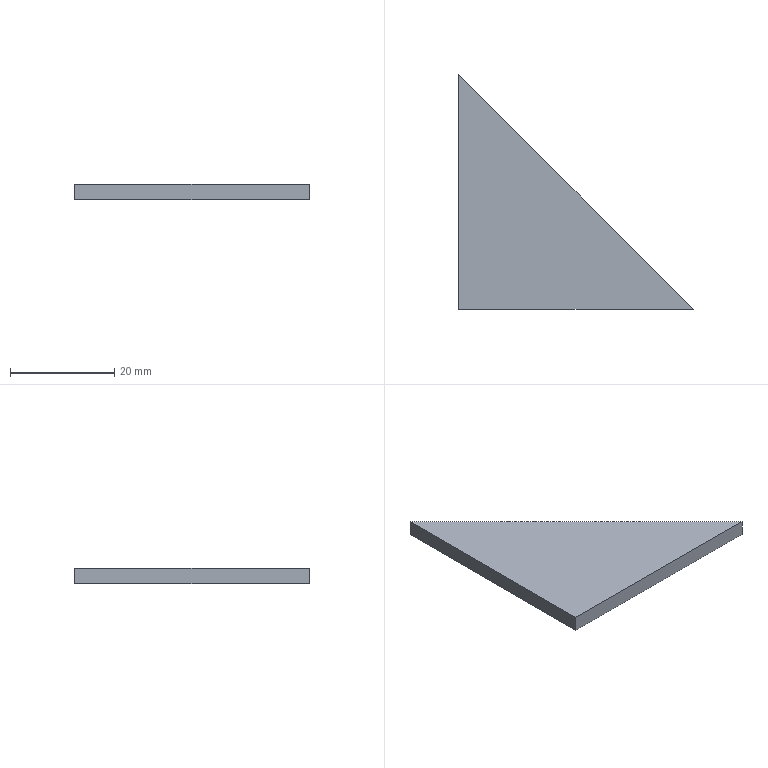Part | STEP file | 5090108 | 1 solid | 5 faces | box 45 x 45 x 3 mm | volume 3037 mm3 | plane 5
STEP:
#1=CARTESIAN_POINT('',(0.,0.,0.));
#2=DIRECTION('',(0.,0.,1.));
#3=DIRECTION('',(1.,0.,0.));
#4=AXIS2_PLACEMENT_3D('',#1,#2,#3);
#5=CARTESIAN_POINT('',(-8.721,-36.279,0.));
#6=VERTEX_POINT('',#5);
#7=CARTESIAN_POINT('',(36.279,-36.279,0.));
#8=VERTEX_POINT('',#7);
#9=CARTESIAN_POINT('',(-8.721,-36.279,0.));
#10=DIRECTION('',(1.,0.,0.));
#11=VECTOR('',#10,1.);
#12=LINE('',#9,#11);
#13=CARTESIAN_POINT('',(-8.721,-36.279,3.));
#14=DIRECTION('',(0.,1.,0.));
#15=DIRECTION('',(0.,0.,1.));
#16=AXIS2_PLACEMENT_3D('',#13,#14,#15);
#17=PLANE('',#16);
#18=CARTESIAN_POINT('',(-3.,0.));
#19=DIRECTION('',(0.,1.));
#20=VECTOR('',#19,1.);
#21=LINE('',#18,#20);
#22=(GEOMETRIC_REPRESENTATION_CONTEXT(2)PARAMETRIC_REPRESENTATION_CONTEXT()REPRESENTATION_CONTEXT('',''));
#23=DEFINITIONAL_REPRESENTATION('',(#21),#22);
#24=PCURVE('',#17,#23);
#25=CARTESIAN_POINT('',(0.,0.,0.));
#26=DIRECTION('',(0.,0.,-1.));
#27=DIRECTION('',(-1.,0.,0.));
#28=AXIS2_PLACEMENT_3D('',#25,#26,#27);
#29=PLANE('',#28);
#30=CARTESIAN_POINT('',(8.721,-36.279));
#31=DIRECTION('',(-1.,0.));
#32=VECTOR('',#31,1.);
#33=LINE('',#30,#32);
#34=(GEOMETRIC_REPRESENTATION_CONTEXT(2)PARAMETRIC_REPRESENTATION_CONTEXT()REPRESENTATION_CONTEXT('',''));
#35=DEFINITIONAL_REPRESENTATION('',(#33),#34);
#36=PCURVE('',#29,#35);
#37=SURFACE_CURVE('',#12,(#24,#36),.PCURVE_S1.);
#38=EDGE_CURVE('',#6,#8,#37,.T.);
#39=ORIENTED_EDGE('',*,*,#38,.T.);
#40=CARTESIAN_POINT('',(36.279,-36.279,3.));
#41=VERTEX_POINT('',#40);
#42=CARTESIAN_POINT('',(36.279,-36.279,3.));
#43=DIRECTION('',(0.,0.,-1.));
#44=VECTOR('',#43,1.);
#45=LINE('',#42,#44);
#46=CARTESIAN_POINT('',(0.,45.));
#47=DIRECTION('',(-1.,0.));
#48=VECTOR('',#47,1.);
#49=LINE('',#46,#48);
#50=(GEOMETRIC_REPRESENTATION_CONTEXT(2)PARAMETRIC_REPRESENTATION_CONTEXT()REPRESENTATION_CONTEXT('',''));
#51=DEFINITIONAL_REPRESENTATION('',(#49),#50);
#52=PCURVE('',#17,#51);
#53=CARTESIAN_POINT('',(-8.721,8.721,3.));
#54=DIRECTION('',(-0.7071,-0.7071,0.));
#55=DIRECTION('',(0.7071,-0.7071,0.));
#56=AXIS2_PLACEMENT_3D('',#53,#54,#55);
#57=PLANE('',#56);
#58=CARTESIAN_POINT('',(63.64,0.));
#59=DIRECTION('',(0.,-1.));
#60=VECTOR('',#59,1.);
#61=LINE('',#58,#60);
#62=(GEOMETRIC_REPRESENTATION_CONTEXT(2)PARAMETRIC_REPRESENTATION_CONTEXT()REPRESENTATION_CONTEXT('',''));
#63=DEFINITIONAL_REPRESENTATION('',(#61),#62);
#64=PCURVE('',#57,#63);
#65=SURFACE_CURVE('',#45,(#52,#64),.PCURVE_S1.);
#66=EDGE_CURVE('',#41,#8,#65,.T.);
#67=ORIENTED_EDGE('',*,*,#66,.F.);
#68=CARTESIAN_POINT('',(-8.721,-36.279,3.));
#69=VERTEX_POINT('',#68);
#70=CARTESIAN_POINT('',(-8.721,-36.279,3.));
#71=DIRECTION('',(1.,0.,0.));
#72=VECTOR('',#71,1.);
#73=LINE('',#70,#72);
#74=CARTESIAN_POINT('',(0.,0.));
#75=DIRECTION('',(0.,1.));
#76=VECTOR('',#75,1.);
#77=LINE('',#74,#76);
#78=(GEOMETRIC_REPRESENTATION_CONTEXT(2)PARAMETRIC_REPRESENTATION_CONTEXT()REPRESENTATION_CONTEXT('',''));
#79=DEFINITIONAL_REPRESENTATION('',(#77),#78);
#80=PCURVE('',#17,#79);
#81=CARTESIAN_POINT('',(0.,0.,3.));
#82=DIRECTION('',(0.,0.,-1.));
#83=DIRECTION('',(-1.,0.,0.));
#84=AXIS2_PLACEMENT_3D('',#81,#82,#83);
#85=PLANE('',#84);
#86=CARTESIAN_POINT('',(8.721,-36.279));
#87=DIRECTION('',(-1.,0.));
#88=VECTOR('',#87,1.);
#89=LINE('',#86,#88);
#90=(GEOMETRIC_REPRESENTATION_CONTEXT(2)PARAMETRIC_REPRESENTATION_CONTEXT()REPRESENTATION_CONTEXT('',''));
#91=DEFINITIONAL_REPRESENTATION('',(#89),#90);
#92=PCURVE('',#85,#91);
#93=SURFACE_CURVE('',#73,(#80,#92),.PCURVE_S1.);
#94=EDGE_CURVE('',#69,#41,#93,.T.);
#95=ORIENTED_EDGE('',*,*,#94,.F.);
#96=CARTESIAN_POINT('',(-8.721,-36.279,3.));
#97=DIRECTION('',(0.,0.,-1.));
#98=VECTOR('',#97,1.);
#99=LINE('',#96,#98);
#100=CARTESIAN_POINT('',(0.,0.));
#101=DIRECTION('',(-1.,0.));
#102=VECTOR('',#101,1.);
#103=LINE('',#100,#102);
#104=(GEOMETRIC_REPRESENTATION_CONTEXT(2)PARAMETRIC_REPRESENTATION_CONTEXT()REPRESENTATION_CONTEXT('',''));
#105=DEFINITIONAL_REPRESENTATION('',(#103),#104);
#106=PCURVE('',#17,#105);
#107=CARTESIAN_POINT('',(-8.721,8.721,3.));
#108=DIRECTION('',(1.,0.,0.));
#109=DIRECTION('',(0.,1.,0.));
#110=AXIS2_PLACEMENT_3D('',#107,#108,#109);
#111=PLANE('',#110);
#112=CARTESIAN_POINT('',(-45.,0.));
#113=DIRECTION('',(0.,-1.));
#114=VECTOR('',#113,1.);
#115=LINE('',#112,#114);
#116=(GEOMETRIC_REPRESENTATION_CONTEXT(2)PARAMETRIC_REPRESENTATION_CONTEXT()REPRESENTATION_CONTEXT('',''));
#117=DEFINITIONAL_REPRESENTATION('',(#115),#116);
#118=PCURVE('',#111,#117);
#119=SURFACE_CURVE('',#99,(#106,#118),.PCURVE_S1.);
#120=EDGE_CURVE('',#69,#6,#119,.T.);
#121=ORIENTED_EDGE('',*,*,#120,.T.);
#122=EDGE_LOOP('',(#39,#67,#95,#121));
#123=FACE_BOUND('',#122,.T.);
#124=ADVANCED_FACE('',(#123),#17,.F.);
#125=CARTESIAN_POINT('',(-8.721,8.721,0.));
#126=VERTEX_POINT('',#125);
#127=CARTESIAN_POINT('',(-8.721,8.721,0.));
#128=DIRECTION('',(-0.7071,0.7071,0.));
#129=VECTOR('',#128,1.);
#130=LINE('',#127,#129);
#131=CARTESIAN_POINT('',(0.,-3.));
#132=DIRECTION('',(-1.,0.));
#133=VECTOR('',#132,1.);
#134=LINE('',#131,#133);
#135=(GEOMETRIC_REPRESENTATION_CONTEXT(2)PARAMETRIC_REPRESENTATION_CONTEXT()REPRESENTATION_CONTEXT('',''));
#136=DEFINITIONAL_REPRESENTATION('',(#134),#135);
#137=PCURVE('',#57,#136);
#138=CARTESIAN_POINT('',(8.721,8.721));
#139=DIRECTION('',(0.7071,0.7071));
#140=VECTOR('',#139,1.);
#141=LINE('',#138,#140);
#142=(GEOMETRIC_REPRESENTATION_CONTEXT(2)PARAMETRIC_REPRESENTATION_CONTEXT()REPRESENTATION_CONTEXT('',''));
#143=DEFINITIONAL_REPRESENTATION('',(#141),#142);
#144=PCURVE('',#29,#143);
#145=SURFACE_CURVE('',#130,(#137,#144),.PCURVE_S1.);
#146=EDGE_CURVE('',#8,#126,#145,.T.);
#147=ORIENTED_EDGE('',*,*,#146,.T.);
#148=CARTESIAN_POINT('',(-8.721,8.721,3.));
#149=VERTEX_POINT('',#148);
#150=CARTESIAN_POINT('',(-8.721,8.721,3.));
#151=DIRECTION('',(0.,0.,-1.));
#152=VECTOR('',#151,1.);
#153=LINE('',#150,#152);
#154=CARTESIAN_POINT('',(0.,0.));
#155=DIRECTION('',(0.,-1.));
#156=VECTOR('',#155,1.);
#157=LINE('',#154,#156);
#158=(GEOMETRIC_REPRESENTATION_CONTEXT(2)PARAMETRIC_REPRESENTATION_CONTEXT()REPRESENTATION_CONTEXT('',''));
#159=DEFINITIONAL_REPRESENTATION('',(#157),#158);
#160=PCURVE('',#57,#159);
#161=CARTESIAN_POINT('',(0.,0.));
#162=DIRECTION('',(0.,-1.));
#163=VECTOR('',#162,1.);
#164=LINE('',#161,#163);
#165=(GEOMETRIC_REPRESENTATION_CONTEXT(2)PARAMETRIC_REPRESENTATION_CONTEXT()REPRESENTATION_CONTEXT('',''));
#166=DEFINITIONAL_REPRESENTATION('',(#164),#165);
#167=PCURVE('',#111,#166);
#168=SURFACE_CURVE('',#153,(#160,#167),.PCURVE_S1.);
#169=EDGE_CURVE('',#149,#126,#168,.T.);
#170=ORIENTED_EDGE('',*,*,#169,.F.);
#171=CARTESIAN_POINT('',(-8.721,8.721,3.));
#172=DIRECTION('',(-0.7071,0.7071,0.));
#173=VECTOR('',#172,1.);
#174=LINE('',#171,#173);
#175=CARTESIAN_POINT('',(0.,0.));
#176=DIRECTION('',(-1.,0.));
#177=VECTOR('',#176,1.);
#178=LINE('',#175,#177);
#179=(GEOMETRIC_REPRESENTATION_CONTEXT(2)PARAMETRIC_REPRESENTATION_CONTEXT()REPRESENTATION_CONTEXT('',''));
#180=DEFINITIONAL_REPRESENTATION('',(#178),#179);
#181=PCURVE('',#57,#180);
#182=CARTESIAN_POINT('',(8.721,8.721));
#183=DIRECTION('',(0.7071,0.7071));
#184=VECTOR('',#183,1.);
#185=LINE('',#182,#184);
#186=(GEOMETRIC_REPRESENTATION_CONTEXT(2)PARAMETRIC_REPRESENTATION_CONTEXT()REPRESENTATION_CONTEXT('',''));
#187=DEFINITIONAL_REPRESENTATION('',(#185),#186);
#188=PCURVE('',#85,#187);
#189=SURFACE_CURVE('',#174,(#181,#188),.PCURVE_S1.);
#190=EDGE_CURVE('',#41,#149,#189,.T.);
#191=ORIENTED_EDGE('',*,*,#190,.F.);
#192=ORIENTED_EDGE('',*,*,#66,.T.);
#193=EDGE_LOOP('',(#147,#170,#191,#192));
#194=FACE_BOUND('',#193,.T.);
#195=ADVANCED_FACE('',(#194),#57,.F.);
#196=CARTESIAN_POINT('',(-8.721,8.721,0.));
#197=DIRECTION('',(0.,-1.,0.));
#198=VECTOR('',#197,1.);
#199=LINE('',#196,#198);
#200=CARTESIAN_POINT('',(0.,-3.));
#201=DIRECTION('',(-1.,0.));
#202=VECTOR('',#201,1.);
#203=LINE('',#200,#202);
#204=(GEOMETRIC_REPRESENTATION_CONTEXT(2)PARAMETRIC_REPRESENTATION_CONTEXT()REPRESENTATION_CONTEXT('',''));
#205=DEFINITIONAL_REPRESENTATION('',(#203),#204);
#206=PCURVE('',#111,#205);
#207=CARTESIAN_POINT('',(8.721,8.721));
#208=DIRECTION('',(0.,-1.));
#209=VECTOR('',#208,1.);
#210=LINE('',#207,#209);
#211=(GEOMETRIC_REPRESENTATION_CONTEXT(2)PARAMETRIC_REPRESENTATION_CONTEXT()REPRESENTATION_CONTEXT('',''));
#212=DEFINITIONAL_REPRESENTATION('',(#210),#211);
#213=PCURVE('',#29,#212);
#214=SURFACE_CURVE('',#199,(#206,#213),.PCURVE_S1.);
#215=EDGE_CURVE('',#126,#6,#214,.T.);
#216=ORIENTED_EDGE('',*,*,#215,.T.);
#217=ORIENTED_EDGE('',*,*,#120,.F.);
#218=CARTESIAN_POINT('',(-8.721,8.721,3.));
#219=DIRECTION('',(0.,-1.,0.));
#220=VECTOR('',#219,1.);
#221=LINE('',#218,#220);
#222=CARTESIAN_POINT('',(0.,0.));
#223=DIRECTION('',(-1.,0.));
#224=VECTOR('',#223,1.);
#225=LINE('',#222,#224);
#226=(GEOMETRIC_REPRESENTATION_CONTEXT(2)PARAMETRIC_REPRESENTATION_CONTEXT()REPRESENTATION_CONTEXT('',''));
#227=DEFINITIONAL_REPRESENTATION('',(#225),#226);
#228=PCURVE('',#111,#227);
#229=CARTESIAN_POINT('',(8.721,8.721));
#230=DIRECTION('',(0.,-1.));
#231=VECTOR('',#230,1.);
#232=LINE('',#229,#231);
#233=(GEOMETRIC_REPRESENTATION_CONTEXT(2)PARAMETRIC_REPRESENTATION_CONTEXT()REPRESENTATION_CONTEXT('',''));
#234=DEFINITIONAL_REPRESENTATION('',(#232),#233);
#235=PCURVE('',#85,#234);
#236=SURFACE_CURVE('',#221,(#228,#235),.PCURVE_S1.);
#237=EDGE_CURVE('',#149,#69,#236,.T.);
#238=ORIENTED_EDGE('',*,*,#237,.F.);
#239=ORIENTED_EDGE('',*,*,#169,.T.);
#240=EDGE_LOOP('',(#216,#217,#238,#239));
#241=FACE_BOUND('',#240,.T.);
#242=ADVANCED_FACE('',(#241),#111,.F.);
#243=ORIENTED_EDGE('',*,*,#94,.T.);
#244=ORIENTED_EDGE('',*,*,#190,.T.);
#245=ORIENTED_EDGE('',*,*,#237,.T.);
#246=EDGE_LOOP('',(#243,#244,#245));
#247=FACE_BOUND('',#246,.T.);
#248=ADVANCED_FACE('',(#247),#85,.F.);
#249=ORIENTED_EDGE('',*,*,#38,.F.);
#250=ORIENTED_EDGE('',*,*,#215,.F.);
#251=ORIENTED_EDGE('',*,*,#146,.F.);
#252=EDGE_LOOP('',(#249,#250,#251));
#253=FACE_BOUND('',#252,.T.);
#254=ADVANCED_FACE('',(#253),#29,.T.);
#255=CLOSED_SHELL('',(#124,#195,#242,#248,#254));
#256=MANIFOLD_SOLID_BREP('',#255);
#257=(LENGTH_UNIT()NAMED_UNIT(*)SI_UNIT(.MILLI.,.METRE.));
#258=UNCERTAINTY_MEASURE_WITH_UNIT(LENGTH_MEASURE(0.0000001),#257,'','');
#259=(NAMED_UNIT(*)PLANE_ANGLE_UNIT()SI_UNIT($,.RADIAN.));
#260=(NAMED_UNIT(*)SI_UNIT($,.STERADIAN.)SOLID_ANGLE_UNIT());
#261=(GEOMETRIC_REPRESENTATION_CONTEXT(3)GLOBAL_UNCERTAINTY_ASSIGNED_CONTEXT((#258))GLOBAL_UNIT_ASSIGNED_CONTEXT((#257,#259,#260))REPRESENTATION_CONTEXT('',''));
#262=ADVANCED_BREP_SHAPE_REPRESENTATION('',(#4,#256),#261);